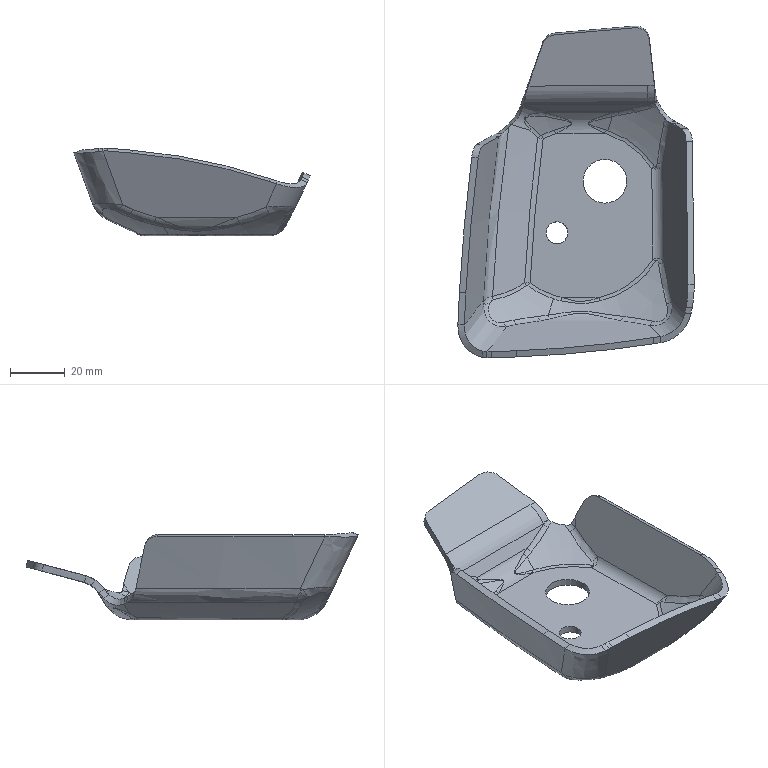Part | 1 solid | 162 faces | box 86.387 x 121.397 x 32.171 mm | volume 27791 mm3 | spline 106 | cylinder 26 | plane 11 | other 11 | torus 8 | commonest cylinder face diameters 19 x6 24 x6 10 x3 8 x2 16 x2 9 x1